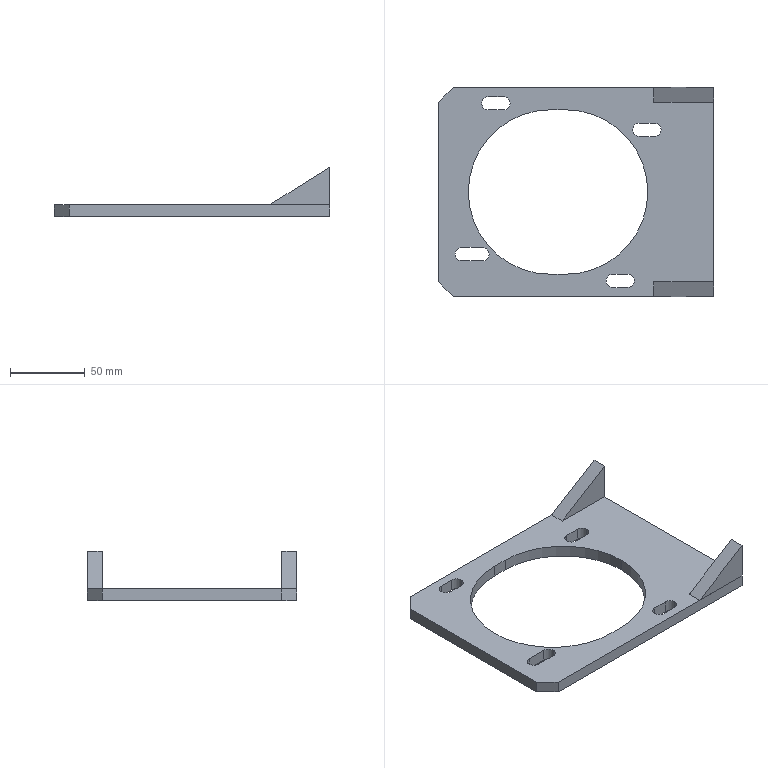Part | STEP file | 3 solids | 43 faces | box 184 x 140 x 33 mm | volume 125268 mm3 | plane 28 | cylinder 15 | commonest cylinder face diameters 9 x12 110 x3